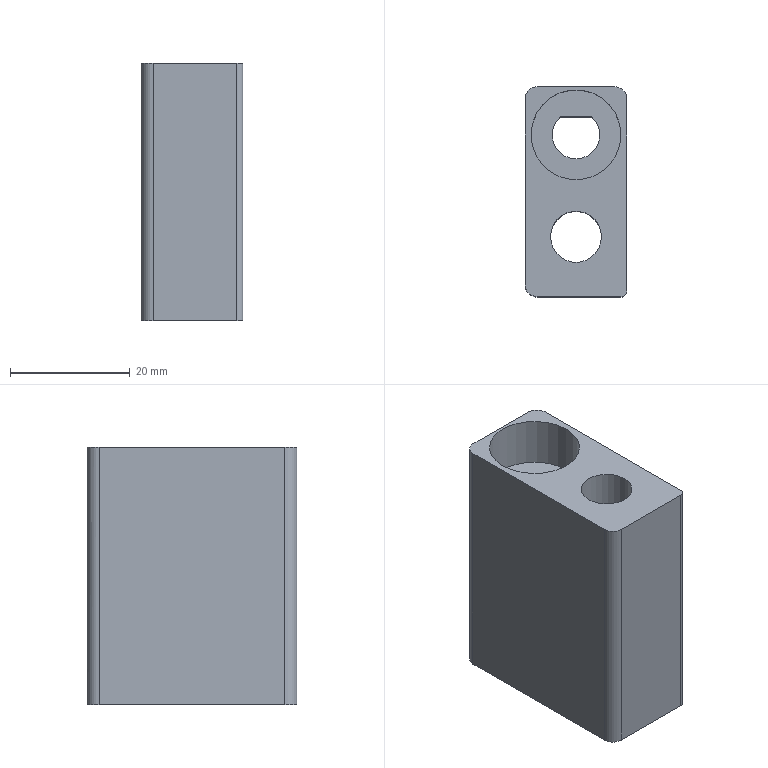Part | NX | features PH-14 2 | 1 solid | 19 faces | box 17 x 35 x 43 mm | volume 18314 mm3 | plane 10 | cylinder 9 | commonest cylinder face diameters 4 x3 2 x1 6.001 x1 8 x1 8.5 x1 14.5 x1
STEP:
#1=CARTESIAN_POINT('',(4095.486,-894.122,902.716));
#2=VERTEX_POINT('',#1);
#3=CARTESIAN_POINT('',(4088.236,-894.122,902.716));
#4=DIRECTION('',(0.,0.,1.));
#5=DIRECTION('',(1.,0.,0.));
#6=AXIS2_PLACEMENT_3D('',#3,#4,#5);
#7=CIRCLE('',#6,7.25);
#8=EDGE_CURVE('',#2,#2,#7,.T.);
#9=ORIENTED_EDGE('',*,*,#8,.T.);
#10=EDGE_LOOP('',(#9));
#11=FACE_BOUND('',#10,.T.);
#12=CARTESIAN_POINT('',(4081.736,-869.122,902.716));
#13=VERTEX_POINT('',#12);
#14=CARTESIAN_POINT('',(4079.736,-871.122,902.716));
#15=VERTEX_POINT('',#14);
#16=CARTESIAN_POINT('',(4081.736,-869.122,902.716));
#17=CARTESIAN_POINT('',(4080.632,-869.122,902.716));
#18=CARTESIAN_POINT('',(4079.736,-870.017,902.716));
#19=CARTESIAN_POINT('',(4079.736,-871.122,902.716));
#20=B_SPLINE_CURVE_WITH_KNOTS('',3,(#16,#17,#18,#19),.UNSPECIFIED.,.F.,.F.,(4,4),(0.,1.),.UNSPECIFIED.);
#21=EDGE_CURVE('',#13,#15,#20,.T.);
#22=ORIENTED_EDGE('',*,*,#21,.F.);
#23=CARTESIAN_POINT('',(4094.736,-869.122,902.716));
#24=VERTEX_POINT('',#23);
#25=CARTESIAN_POINT('',(4088.236,-869.122,902.716));
#26=DIRECTION('',(-1.,0.,0.));
#27=VECTOR('',#26,1000.);
#28=LINE('',#25,#27);
#29=EDGE_CURVE('',#24,#13,#28,.T.);
#30=ORIENTED_EDGE('',*,*,#29,.F.);
#31=CARTESIAN_POINT('',(4096.736,-871.122,902.716));
#32=VERTEX_POINT('',#31);
#33=CARTESIAN_POINT('',(4094.736,-871.122,902.716));
#34=DIRECTION('',(0.,0.,-1.));
#35=DIRECTION('',(-1.,0.,0.));
#36=AXIS2_PLACEMENT_3D('',#33,#34,#35);
#37=CIRCLE('',#36,2.);
#38=EDGE_CURVE('',#32,#24,#37,.F.);
#39=ORIENTED_EDGE('',*,*,#38,.F.);
#40=CARTESIAN_POINT('',(4096.736,-903.122,902.716));
#41=VERTEX_POINT('',#40);
#42=CARTESIAN_POINT('',(4096.736,-886.622,902.716));
#43=DIRECTION('',(0.,1.,0.));
#44=VECTOR('',#43,1000.);
#45=LINE('',#42,#44);
#46=EDGE_CURVE('',#41,#32,#45,.T.);
#47=ORIENTED_EDGE('',*,*,#46,.F.);
#48=CARTESIAN_POINT('',(4095.736,-904.122,902.716));
#49=VERTEX_POINT('',#48);
#50=CARTESIAN_POINT('',(4095.736,-903.122,902.716));
#51=DIRECTION('',(0.,0.,-1.));
#52=DIRECTION('',(-1.,0.,0.));
#53=AXIS2_PLACEMENT_3D('',#50,#51,#52);
#54=CIRCLE('',#53,1.);
#55=EDGE_CURVE('',#41,#49,#54,.T.);
#56=ORIENTED_EDGE('',*,*,#55,.T.);
#57=CARTESIAN_POINT('',(4081.736,-904.122,902.716));
#58=VERTEX_POINT('',#57);
#59=CARTESIAN_POINT('',(4088.236,-904.122,902.716));
#60=DIRECTION('',(1.,0.,0.));
#61=VECTOR('',#60,1000.);
#62=LINE('',#59,#61);
#63=EDGE_CURVE('',#58,#49,#62,.T.);
#64=ORIENTED_EDGE('',*,*,#63,.F.);
#65=CARTESIAN_POINT('',(4079.736,-902.122,902.716));
#66=VERTEX_POINT('',#65);
#67=CARTESIAN_POINT('',(4081.736,-902.122,902.716));
#68=DIRECTION('',(0.,0.,-1.));
#69=DIRECTION('',(-1.,0.,0.));
#70=AXIS2_PLACEMENT_3D('',#67,#68,#69);
#71=CIRCLE('',#70,2.);
#72=EDGE_CURVE('',#66,#58,#71,.F.);
#73=ORIENTED_EDGE('',*,*,#72,.F.);
#74=CARTESIAN_POINT('',(4079.736,-886.622,902.716));
#75=DIRECTION('',(0.,1.,0.));
#76=VECTOR('',#75,1000.);
#77=LINE('',#74,#76);
#78=EDGE_CURVE('',#66,#15,#77,.T.);
#79=ORIENTED_EDGE('',*,*,#78,.T.);
#80=EDGE_LOOP('',(#22,#30,#39,#47,#56,#64,#73,#79));
#81=FACE_BOUND('',#80,.T.);
#82=CARTESIAN_POINT('',(4090.882,-874.122,902.716));
#83=VERTEX_POINT('',#82);
#84=CARTESIAN_POINT('',(4085.59,-874.122,902.716));
#85=VERTEX_POINT('',#84);
#86=CARTESIAN_POINT('',(4088.236,-877.122,902.716));
#87=DIRECTION('',(0.,0.,-1.));
#88=DIRECTION('',(-1.,0.,0.));
#89=AXIS2_PLACEMENT_3D('',#86,#87,#88);
#90=CIRCLE('',#89,4.);
#91=EDGE_CURVE('',#83,#85,#90,.T.);
#92=ORIENTED_EDGE('',*,*,#91,.F.);
#93=CARTESIAN_POINT('',(4088.285,-874.122,902.716));
#94=VERTEX_POINT('',#93);
#95=CARTESIAN_POINT('',(4079.736,-874.122,902.716));
#96=DIRECTION('',(-1.,0.,0.));
#97=VECTOR('',#96,1000.);
#98=LINE('',#95,#97);
#99=EDGE_CURVE('',#83,#94,#98,.T.);
#100=ORIENTED_EDGE('',*,*,#99,.T.);
#101=CARTESIAN_POINT('',(4088.187,-874.122,902.716));
#102=VERTEX_POINT('',#101);
#103=CARTESIAN_POINT('',(4088.236,-877.122,902.716));
#104=DIRECTION('',(0.,0.,-1.));
#105=DIRECTION('',(-1.,0.,0.));
#106=AXIS2_PLACEMENT_3D('',#103,#104,#105);
#107=CIRCLE('',#106,3.);
#108=EDGE_CURVE('',#102,#94,#107,.T.);
#109=ORIENTED_EDGE('',*,*,#108,.F.);
#110=CARTESIAN_POINT('',(4079.736,-874.122,902.716));
#111=DIRECTION('',(-1.,0.,0.));
#112=VECTOR('',#111,1000.);
#113=LINE('',#110,#112);
#114=EDGE_CURVE('',#102,#85,#113,.T.);
#115=ORIENTED_EDGE('',*,*,#114,.T.);
#116=EDGE_LOOP('',(#92,#100,#109,#115));
#117=FACE_BOUND('',#116,.T.);
#118=CARTESIAN_POINT('',(4079.736,-888.622,902.716));
#119=DIRECTION('',(0.,0.,-1.));
#120=DIRECTION('',(1.,0.,0.));
#121=AXIS2_PLACEMENT_3D('',#118,#119,#120);
#122=PLANE('',#121);
#123=ADVANCED_FACE('',(#11,#81,#117),#122,.T.);
#124=CARTESIAN_POINT('',(4088.187,-874.122,937.416));
#125=VERTEX_POINT('',#124);
#126=CARTESIAN_POINT('',(4088.187,-874.122,945.716));
#127=DIRECTION('',(0.,0.,-1.));
#128=VECTOR('',#127,1000.);
#129=LINE('',#126,#128);
#130=EDGE_CURVE('',#102,#125,#129,.F.);
#131=ORIENTED_EDGE('',*,*,#130,.F.);
#132=ORIENTED_EDGE('',*,*,#108,.T.);
#133=CARTESIAN_POINT('',(4088.285,-874.122,937.416));
#134=VERTEX_POINT('',#133);
#135=CARTESIAN_POINT('',(4088.285,-874.122,945.716));
#136=DIRECTION('',(0.,0.,-1.));
#137=VECTOR('',#136,1000.);
#138=LINE('',#135,#137);
#139=EDGE_CURVE('',#134,#94,#138,.T.);
#140=ORIENTED_EDGE('',*,*,#139,.F.);
#141=CARTESIAN_POINT('',(4088.236,-877.122,937.416));
#142=DIRECTION('',(0.,0.,-1.));
#143=DIRECTION('',(-1.,0.,0.));
#144=AXIS2_PLACEMENT_3D('',#141,#142,#143);
#145=CIRCLE('',#144,3.);
#146=EDGE_CURVE('',#125,#134,#145,.T.);
#147=ORIENTED_EDGE('',*,*,#146,.F.);
#148=EDGE_LOOP('',(#131,#132,#140,#147));
#149=FACE_BOUND('',#148,.T.);
#150=CARTESIAN_POINT('',(4088.236,-877.122,945.716));
#151=DIRECTION('',(0.,0.,-1.));
#152=DIRECTION('',(1.,0.,0.));
#153=AXIS2_PLACEMENT_3D('',#150,#151,#152);
#154=CYLINDRICAL_SURFACE('',#153,3.);
#155=ADVANCED_FACE('',(#149),#154,.F.);
#156=CARTESIAN_POINT('',(4080.736,-877.122,937.416));
#157=VERTEX_POINT('',#156);
#158=CARTESIAN_POINT('',(4088.236,-877.122,937.416));
#159=DIRECTION('',(0.,0.,-1.));
#160=DIRECTION('',(-1.,0.,0.));
#161=AXIS2_PLACEMENT_3D('',#158,#159,#160);
#162=CIRCLE('',#161,7.5);
#163=EDGE_CURVE('',#157,#157,#162,.T.);
#164=ORIENTED_EDGE('',*,*,#163,.F.);
#165=EDGE_LOOP('',(#164));
#166=FACE_BOUND('',#165,.T.);
#167=CARTESIAN_POINT('',(4090.882,-874.122,937.416));
#168=VERTEX_POINT('',#167);
#169=CARTESIAN_POINT('',(4088.236,-874.122,937.416));
#170=DIRECTION('',(-1.,0.,0.));
#171=VECTOR('',#170,1000.);
#172=LINE('',#169,#171);
#173=EDGE_CURVE('',#168,#134,#172,.T.);
#174=ORIENTED_EDGE('',*,*,#173,.F.);
#175=CARTESIAN_POINT('',(4085.59,-874.122,937.416));
#176=VERTEX_POINT('',#175);
#177=CARTESIAN_POINT('',(4088.236,-877.122,937.416));
#178=DIRECTION('',(0.,0.,-1.));
#179=DIRECTION('',(-1.,0.,0.));
#180=AXIS2_PLACEMENT_3D('',#177,#178,#179);
#181=CIRCLE('',#180,4.);
#182=EDGE_CURVE('',#168,#176,#181,.T.);
#183=ORIENTED_EDGE('',*,*,#182,.T.);
#184=CARTESIAN_POINT('',(4088.236,-874.122,937.416));
#185=DIRECTION('',(-1.,0.,0.));
#186=VECTOR('',#185,1000.);
#187=LINE('',#184,#186);
#188=EDGE_CURVE('',#125,#176,#187,.T.);
#189=ORIENTED_EDGE('',*,*,#188,.F.);
#190=ORIENTED_EDGE('',*,*,#146,.T.);
#191=EDGE_LOOP('',(#174,#183,#189,#190));
#192=FACE_BOUND('',#191,.T.);
#193=CARTESIAN_POINT('',(4088.236,-877.122,937.416));
#194=DIRECTION('',(0.,0.,-1.));
#195=DIRECTION('',(-1.,0.,0.));
#196=AXIS2_PLACEMENT_3D('',#193,#194,#195);
#197=PLANE('',#196);
#198=ADVANCED_FACE('',(#166,#192),#197,.F.);
#199=CARTESIAN_POINT('',(4092.486,-894.122,945.716));
#200=VERTEX_POINT('',#199);
#201=CARTESIAN_POINT('',(4088.236,-894.122,945.716));
#202=DIRECTION('',(0.,0.,1.));
#203=DIRECTION('',(1.,0.,0.));
#204=AXIS2_PLACEMENT_3D('',#201,#202,#203);
#205=CIRCLE('',#204,4.25);
#206=EDGE_CURVE('',#200,#200,#205,.T.);
#207=ORIENTED_EDGE('',*,*,#206,.F.);
#208=EDGE_LOOP('',(#207));
#209=FACE_BOUND('',#208,.T.);
#210=CARTESIAN_POINT('',(4079.736,-871.122,945.716));
#211=VERTEX_POINT('',#210);
#212=CARTESIAN_POINT('',(4081.736,-869.122,945.716));
#213=VERTEX_POINT('',#212);
#214=CARTESIAN_POINT('',(4079.736,-871.122,945.716));
#215=CARTESIAN_POINT('',(4079.736,-870.018,945.716));
#216=CARTESIAN_POINT('',(4080.631,-869.122,945.716));
#217=CARTESIAN_POINT('',(4081.736,-869.122,945.716));
#218=B_SPLINE_CURVE_WITH_KNOTS('',3,(#214,#215,#216,#217),.UNSPECIFIED.,.F.,.F.,(4,4),(0.,1.),.UNSPECIFIED.);
#219=EDGE_CURVE('',#211,#213,#218,.T.);
#220=ORIENTED_EDGE('',*,*,#219,.F.);
#221=CARTESIAN_POINT('',(4079.736,-902.122,945.716));
#222=VERTEX_POINT('',#221);
#223=CARTESIAN_POINT('',(4079.736,-886.622,945.716));
#224=DIRECTION('',(0.,-1.,0.));
#225=VECTOR('',#224,1000.);
#226=LINE('',#223,#225);
#227=EDGE_CURVE('',#211,#222,#226,.T.);
#228=ORIENTED_EDGE('',*,*,#227,.T.);
#229=CARTESIAN_POINT('',(4081.736,-904.122,945.716));
#230=VERTEX_POINT('',#229);
#231=CARTESIAN_POINT('',(4081.736,-902.122,945.716));
#232=DIRECTION('',(0.,0.,1.));
#233=DIRECTION('',(1.,0.,0.));
#234=AXIS2_PLACEMENT_3D('',#231,#232,#233);
#235=CIRCLE('',#234,2.);
#236=EDGE_CURVE('',#230,#222,#235,.F.);
#237=ORIENTED_EDGE('',*,*,#236,.F.);
#238=CARTESIAN_POINT('',(4095.736,-904.122,945.716));
#239=VERTEX_POINT('',#238);
#240=CARTESIAN_POINT('',(4088.236,-904.122,945.716));
#241=DIRECTION('',(-1.,0.,0.));
#242=VECTOR('',#241,1000.);
#243=LINE('',#240,#242);
#244=EDGE_CURVE('',#239,#230,#243,.T.);
#245=ORIENTED_EDGE('',*,*,#244,.F.);
#246=CARTESIAN_POINT('',(4096.736,-903.122,945.716));
#247=VERTEX_POINT('',#246);
#248=CARTESIAN_POINT('',(4095.736,-903.122,945.716));
#249=DIRECTION('',(0.,0.,1.));
#250=DIRECTION('',(1.,0.,0.));
#251=AXIS2_PLACEMENT_3D('',#248,#249,#250);
#252=CIRCLE('',#251,1.);
#253=EDGE_CURVE('',#247,#239,#252,.F.);
#254=ORIENTED_EDGE('',*,*,#253,.F.);
#255=CARTESIAN_POINT('',(4096.736,-871.122,945.716));
#256=VERTEX_POINT('',#255);
#257=CARTESIAN_POINT('',(4096.736,-886.622,945.716));
#258=DIRECTION('',(0.,-1.,0.));
#259=VECTOR('',#258,1000.);
#260=LINE('',#257,#259);
#261=EDGE_CURVE('',#256,#247,#260,.T.);
#262=ORIENTED_EDGE('',*,*,#261,.F.);
#263=CARTESIAN_POINT('',(4094.736,-869.122,945.716));
#264=VERTEX_POINT('',#263);
#265=CARTESIAN_POINT('',(4094.736,-871.122,945.716));
#266=DIRECTION('',(0.,0.,1.));
#267=DIRECTION('',(1.,0.,0.));
#268=AXIS2_PLACEMENT_3D('',#265,#266,#267);
#269=CIRCLE('',#268,2.);
#270=EDGE_CURVE('',#264,#256,#269,.F.);
#271=ORIENTED_EDGE('',*,*,#270,.F.);
#272=CARTESIAN_POINT('',(4088.236,-869.122,945.716));
#273=DIRECTION('',(1.,0.,0.));
#274=VECTOR('',#273,1000.);
#275=LINE('',#272,#274);
#276=EDGE_CURVE('',#213,#264,#275,.T.);
#277=ORIENTED_EDGE('',*,*,#276,.F.);
#278=EDGE_LOOP('',(#220,#228,#237,#245,#254,#262,#271,#277));
#279=FACE_BOUND('',#278,.T.);
#280=CARTESIAN_POINT('',(4095.736,-877.122,945.716));
#281=VERTEX_POINT('',#280);
#282=CARTESIAN_POINT('',(4088.236,-877.122,945.716));
#283=DIRECTION('',(0.,0.,1.));
#284=DIRECTION('',(1.,0.,0.));
#285=AXIS2_PLACEMENT_3D('',#282,#283,#284);
#286=CIRCLE('',#285,7.5);
#287=EDGE_CURVE('',#281,#281,#286,.F.);
#288=ORIENTED_EDGE('',*,*,#287,.T.);
#289=EDGE_LOOP('',(#288));
#290=FACE_BOUND('',#289,.T.);
#291=CARTESIAN_POINT('',(4079.736,-888.622,945.716));
#292=DIRECTION('',(0.,0.,1.));
#293=DIRECTION('',(-1.,0.,0.));
#294=AXIS2_PLACEMENT_3D('',#291,#292,#293);
#295=PLANE('',#294);
#296=ADVANCED_FACE('',(#209,#279,#290),#295,.T.);
#297=ORIENTED_EDGE('',*,*,#163,.T.);
#298=EDGE_LOOP('',(#297));
#299=FACE_BOUND('',#298,.T.);
#300=ORIENTED_EDGE('',*,*,#287,.F.);
#301=EDGE_LOOP('',(#300));
#302=FACE_BOUND('',#301,.T.);
#303=CARTESIAN_POINT('',(4088.236,-877.122,945.716));
#304=DIRECTION('',(0.,0.,-1.));
#305=DIRECTION('',(1.,0.,0.));
#306=AXIS2_PLACEMENT_3D('',#303,#304,#305);
#307=CYLINDRICAL_SURFACE('',#306,7.5);
#308=ADVANCED_FACE('',(#299,#302),#307,.F.);
#309=ORIENTED_EDGE('',*,*,#91,.T.);
#310=CARTESIAN_POINT('',(4085.59,-874.122,940.716));
#311=DIRECTION('',(0.,0.,-1.));
#312=VECTOR('',#311,1000.);
#313=LINE('',#310,#312);
#314=EDGE_CURVE('',#176,#85,#313,.T.);
#315=ORIENTED_EDGE('',*,*,#314,.F.);
#316=ORIENTED_EDGE('',*,*,#182,.F.);
#317=CARTESIAN_POINT('',(4090.882,-874.122,940.716));
#318=DIRECTION('',(0.,0.,-1.));
#319=VECTOR('',#318,1000.);
#320=LINE('',#317,#319);
#321=EDGE_CURVE('',#83,#168,#320,.F.);
#322=ORIENTED_EDGE('',*,*,#321,.F.);
#323=EDGE_LOOP('',(#309,#315,#316,#322));
#324=FACE_BOUND('',#323,.T.);
#325=CARTESIAN_POINT('',(4088.236,-877.122,940.716));
#326=DIRECTION('',(0.,0.,-1.));
#327=DIRECTION('',(-1.,0.,0.));
#328=AXIS2_PLACEMENT_3D('',#325,#326,#327);
#329=CYLINDRICAL_SURFACE('',#328,4.);
#330=ADVANCED_FACE('',(#324),#329,.F.);
#331=ORIENTED_EDGE('',*,*,#321,.T.);
#332=ORIENTED_EDGE('',*,*,#173,.T.);
#333=ORIENTED_EDGE('',*,*,#139,.T.);
#334=ORIENTED_EDGE('',*,*,#99,.F.);
#335=EDGE_LOOP('',(#331,#332,#333,#334));
#336=FACE_BOUND('',#335,.T.);
#337=CARTESIAN_POINT('',(4081.317,-874.122,940.716));
#338=DIRECTION('',(0.,-1.,0.));
#339=DIRECTION('',(1.,0.,0.));
#340=AXIS2_PLACEMENT_3D('',#337,#338,#339);
#341=PLANE('',#340);
#342=ADVANCED_FACE('',(#336),#341,.T.);
#343=ORIENTED_EDGE('',*,*,#130,.T.);
#344=ORIENTED_EDGE('',*,*,#188,.T.);
#345=ORIENTED_EDGE('',*,*,#314,.T.);
#346=ORIENTED_EDGE('',*,*,#114,.F.);
#347=EDGE_LOOP('',(#343,#344,#345,#346));
#348=FACE_BOUND('',#347,.T.);
#349=CARTESIAN_POINT('',(4081.317,-874.122,940.716));
#350=DIRECTION('',(0.,-1.,0.));
#351=DIRECTION('',(1.,0.,0.));
#352=AXIS2_PLACEMENT_3D('',#349,#350,#351);
#353=PLANE('',#352);
#354=ADVANCED_FACE('',(#348),#353,.T.);
#355=CARTESIAN_POINT('',(4079.736,-902.122,915.716));
#356=DIRECTION('',(0.,0.,1.));
#357=VECTOR('',#356,1000.);
#358=LINE('',#355,#357);
#359=EDGE_CURVE('',#222,#66,#358,.F.);
#360=ORIENTED_EDGE('',*,*,#359,.F.);
#361=ORIENTED_EDGE('',*,*,#227,.F.);
#362=CARTESIAN_POINT('',(4079.736,-871.122,915.716));
#363=DIRECTION('',(0.,0.,1.));
#364=VECTOR('',#363,1000.);
#365=LINE('',#362,#364);
#366=EDGE_CURVE('',#211,#15,#365,.F.);
#367=ORIENTED_EDGE('',*,*,#366,.T.);
#368=ORIENTED_EDGE('',*,*,#78,.F.);
#369=EDGE_LOOP('',(#360,#361,#367,#368));
#370=FACE_BOUND('',#369,.T.);
#371=CARTESIAN_POINT('',(4079.736,-886.622,915.716));
#372=DIRECTION('',(1.,0.,0.));
#373=DIRECTION('',(0.,0.,1.));
#374=AXIS2_PLACEMENT_3D('',#371,#372,#373);
#375=PLANE('',#374);
#376=ADVANCED_FACE('',(#370),#375,.F.);
#377=ORIENTED_EDGE('',*,*,#55,.F.);
#378=CARTESIAN_POINT('',(4096.736,-903.122,915.716));
#379=DIRECTION('',(0.,0.,1.));
#380=VECTOR('',#379,1000.);
#381=LINE('',#378,#380);
#382=EDGE_CURVE('',#247,#41,#381,.F.);
#383=ORIENTED_EDGE('',*,*,#382,.F.);
#384=ORIENTED_EDGE('',*,*,#253,.T.);
#385=CARTESIAN_POINT('',(4095.736,-904.122,915.716));
#386=DIRECTION('',(0.,0.,1.));
#387=VECTOR('',#386,1000.);
#388=LINE('',#385,#387);
#389=EDGE_CURVE('',#49,#239,#388,.T.);
#390=ORIENTED_EDGE('',*,*,#389,.F.);
#391=EDGE_LOOP('',(#377,#383,#384,#390));
#392=FACE_BOUND('',#391,.T.);
#393=CARTESIAN_POINT('',(4095.736,-903.122,915.716));
#394=DIRECTION('',(0.,0.,1.));
#395=DIRECTION('',(1.,0.,0.));
#396=AXIS2_PLACEMENT_3D('',#393,#394,#395);
#397=CYLINDRICAL_SURFACE('',#396,1.);
#398=ADVANCED_FACE('',(#392),#397,.T.);
#399=ORIENTED_EDGE('',*,*,#38,.T.);
#400=CARTESIAN_POINT('',(4094.736,-869.122,915.716));
#401=DIRECTION('',(0.,0.,1.));
#402=VECTOR('',#401,1000.);
#403=LINE('',#400,#402);
#404=EDGE_CURVE('',#264,#24,#403,.F.);
#405=ORIENTED_EDGE('',*,*,#404,.F.);
#406=ORIENTED_EDGE('',*,*,#270,.T.);
#407=CARTESIAN_POINT('',(4096.736,-871.122,915.716));
#408=DIRECTION('',(0.,0.,1.));
#409=VECTOR('',#408,1000.);
#410=LINE('',#407,#409);
#411=EDGE_CURVE('',#32,#256,#410,.T.);
#412=ORIENTED_EDGE('',*,*,#411,.F.);
#413=EDGE_LOOP('',(#399,#405,#406,#412));
#414=FACE_BOUND('',#413,.T.);
#415=CARTESIAN_POINT('',(4094.736,-871.122,915.716));
#416=DIRECTION('',(0.,0.,1.));
#417=DIRECTION('',(1.,0.,0.));
#418=AXIS2_PLACEMENT_3D('',#415,#416,#417);
#419=CYLINDRICAL_SURFACE('',#418,2.);
#420=ADVANCED_FACE('',(#414),#419,.T.);
#421=ORIENTED_EDGE('',*,*,#72,.T.);
#422=CARTESIAN_POINT('',(4081.736,-904.122,915.716));
#423=DIRECTION('',(0.,0.,1.));
#424=VECTOR('',#423,1000.);
#425=LINE('',#422,#424);
#426=EDGE_CURVE('',#230,#58,#425,.F.);
#427=ORIENTED_EDGE('',*,*,#426,.F.);
#428=ORIENTED_EDGE('',*,*,#236,.T.);
#429=ORIENTED_EDGE('',*,*,#359,.T.);
#430=EDGE_LOOP('',(#421,#427,#428,#429));
#431=FACE_BOUND('',#430,.T.);
#432=CARTESIAN_POINT('',(4081.736,-902.122,915.716));
#433=DIRECTION('',(0.,0.,1.));
#434=DIRECTION('',(1.,0.,0.));
#435=AXIS2_PLACEMENT_3D('',#432,#433,#434);
#436=CYLINDRICAL_SURFACE('',#435,2.);
#437=ADVANCED_FACE('',(#431),#436,.T.);
#438=ORIENTED_EDGE('',*,*,#63,.T.);
#439=ORIENTED_EDGE('',*,*,#389,.T.);
#440=ORIENTED_EDGE('',*,*,#244,.T.);
#441=ORIENTED_EDGE('',*,*,#426,.T.);
#442=EDGE_LOOP('',(#438,#439,#440,#441));
#443=FACE_BOUND('',#442,.T.);
#444=CARTESIAN_POINT('',(4088.236,-904.122,915.716));
#445=DIRECTION('',(0.,-1.,0.));
#446=DIRECTION('',(0.,0.,1.));
#447=AXIS2_PLACEMENT_3D('',#444,#445,#446);
#448=PLANE('',#447);
#449=ADVANCED_FACE('',(#443),#448,.T.);
#450=ORIENTED_EDGE('',*,*,#261,.T.);
#451=ORIENTED_EDGE('',*,*,#382,.T.);
#452=ORIENTED_EDGE('',*,*,#46,.T.);
#453=ORIENTED_EDGE('',*,*,#411,.T.);
#454=EDGE_LOOP('',(#450,#451,#452,#453));
#455=FACE_BOUND('',#454,.T.);
#456=CARTESIAN_POINT('',(4096.736,-886.622,915.716));
#457=DIRECTION('',(1.,0.,0.));
#458=DIRECTION('',(0.,0.,1.));
#459=AXIS2_PLACEMENT_3D('',#456,#457,#458);
#460=PLANE('',#459);
#461=ADVANCED_FACE('',(#455),#460,.T.);
#462=ORIENTED_EDGE('',*,*,#21,.T.);
#463=ORIENTED_EDGE('',*,*,#366,.F.);
#464=ORIENTED_EDGE('',*,*,#219,.T.);
#465=CARTESIAN_POINT('',(4081.736,-869.122,915.716));
#466=DIRECTION('',(0.,0.,1.));
#467=VECTOR('',#466,1000.);
#468=LINE('',#465,#467);
#469=EDGE_CURVE('',#13,#213,#468,.T.);
#470=ORIENTED_EDGE('',*,*,#469,.F.);
#471=EDGE_LOOP('',(#462,#463,#464,#470));
#472=FACE_BOUND('',#471,.T.);
#473=CARTESIAN_POINT('',(4081.736,-871.122,915.716));
#474=DIRECTION('',(0.,0.,1.));
#475=DIRECTION('',(1.,0.,0.));
#476=AXIS2_PLACEMENT_3D('',#473,#474,#475);
#477=CYLINDRICAL_SURFACE('',#476,2.);
#478=ADVANCED_FACE('',(#472),#477,.T.);
#479=ORIENTED_EDGE('',*,*,#29,.T.);
#480=ORIENTED_EDGE('',*,*,#469,.T.);
#481=ORIENTED_EDGE('',*,*,#276,.T.);
#482=ORIENTED_EDGE('',*,*,#404,.T.);
#483=EDGE_LOOP('',(#479,#480,#481,#482));
#484=FACE_BOUND('',#483,.T.);
#485=CARTESIAN_POINT('',(4088.236,-869.122,915.716));
#486=DIRECTION('',(0.,1.,0.));
#487=DIRECTION('',(0.,0.,-1.));
#488=AXIS2_PLACEMENT_3D('',#485,#486,#487);
#489=PLANE('',#488);
#490=ADVANCED_FACE('',(#484),#489,.T.);
#491=ORIENTED_EDGE('',*,*,#206,.T.);
#492=EDGE_LOOP('',(#491));
#493=FACE_BOUND('',#492,.T.);
#494=CARTESIAN_POINT('',(4092.486,-894.122,917.716));
#495=VERTEX_POINT('',#494);
#496=CARTESIAN_POINT('',(4088.236,-894.122,917.716));
#497=DIRECTION('',(0.,0.,1.));
#498=DIRECTION('',(1.,0.,0.));
#499=AXIS2_PLACEMENT_3D('',#496,#497,#498);
#500=CIRCLE('',#499,4.25);
#501=EDGE_CURVE('',#495,#495,#500,.T.);
#502=ORIENTED_EDGE('',*,*,#501,.F.);
#503=EDGE_LOOP('',(#502));
#504=FACE_BOUND('',#503,.T.);
#505=CARTESIAN_POINT('',(4088.236,-894.122,902.716));
#506=DIRECTION('',(0.,0.,1.));
#507=DIRECTION('',(1.,0.,0.));
#508=AXIS2_PLACEMENT_3D('',#505,#506,#507);
#509=CYLINDRICAL_SURFACE('',#508,4.25);
#510=ADVANCED_FACE('',(#493,#504),#509,.F.);
#511=ORIENTED_EDGE('',*,*,#501,.T.);
#512=EDGE_LOOP('',(#511));
#513=FACE_BOUND('',#512,.T.);
#514=CARTESIAN_POINT('',(4095.486,-894.122,917.716));
#515=VERTEX_POINT('',#514);
#516=CARTESIAN_POINT('',(4088.236,-894.122,917.716));
#517=DIRECTION('',(0.,0.,-1.));
#518=DIRECTION('',(1.,0.,0.));
#519=AXIS2_PLACEMENT_3D('',#516,#517,#518);
#520=CIRCLE('',#519,7.25);
#521=EDGE_CURVE('',#515,#515,#520,.F.);
#522=ORIENTED_EDGE('',*,*,#521,.F.);
#523=EDGE_LOOP('',(#522));
#524=FACE_BOUND('',#523,.T.);
#525=CARTESIAN_POINT('',(4088.236,-894.122,917.716));
#526=DIRECTION('',(0.,0.,1.));
#527=DIRECTION('',(1.,0.,0.));
#528=AXIS2_PLACEMENT_3D('',#525,#526,#527);
#529=PLANE('',#528);
#530=ADVANCED_FACE('',(#513,#524),#529,.F.);
#531=ORIENTED_EDGE('',*,*,#521,.T.);
#532=EDGE_LOOP('',(#531));
#533=FACE_BOUND('',#532,.T.);
#534=ORIENTED_EDGE('',*,*,#8,.F.);
#535=EDGE_LOOP('',(#534));
#536=FACE_BOUND('',#535,.T.);
#537=CARTESIAN_POINT('',(4088.236,-894.122,902.716));
#538=DIRECTION('',(0.,0.,1.));
#539=DIRECTION('',(1.,0.,0.));
#540=AXIS2_PLACEMENT_3D('',#537,#538,#539);
#541=CYLINDRICAL_SURFACE('',#540,7.25);
#542=ADVANCED_FACE('',(#533,#536),#541,.F.);
#543=CLOSED_SHELL('',(#123,#155,#198,#296,#308,#330,#342,#354,#376,#398,#420,#437,#449,#461,#478,#490,#510,#530,#542));
#544=MANIFOLD_SOLID_BREP('',#543);
#545=(LENGTH_UNIT()NAMED_UNIT(*)SI_UNIT(.MILLI.,.METRE.));
#546=UNCERTAINTY_MEASURE_WITH_UNIT(LENGTH_MEASURE(0.0508),#545,'','');
#547=(NAMED_UNIT(*)PLANE_ANGLE_UNIT()SI_UNIT($,.RADIAN.));
#548=(NAMED_UNIT(*)SI_UNIT($,.STERADIAN.)SOLID_ANGLE_UNIT());
#549=(GEOMETRIC_REPRESENTATION_CONTEXT(3)GLOBAL_UNCERTAINTY_ASSIGNED_CONTEXT((#546))GLOBAL_UNIT_ASSIGNED_CONTEXT((#545,#547,#548))REPRESENTATION_CONTEXT('',''));
#550=ADVANCED_BREP_SHAPE_REPRESENTATION('',(#544),#549);